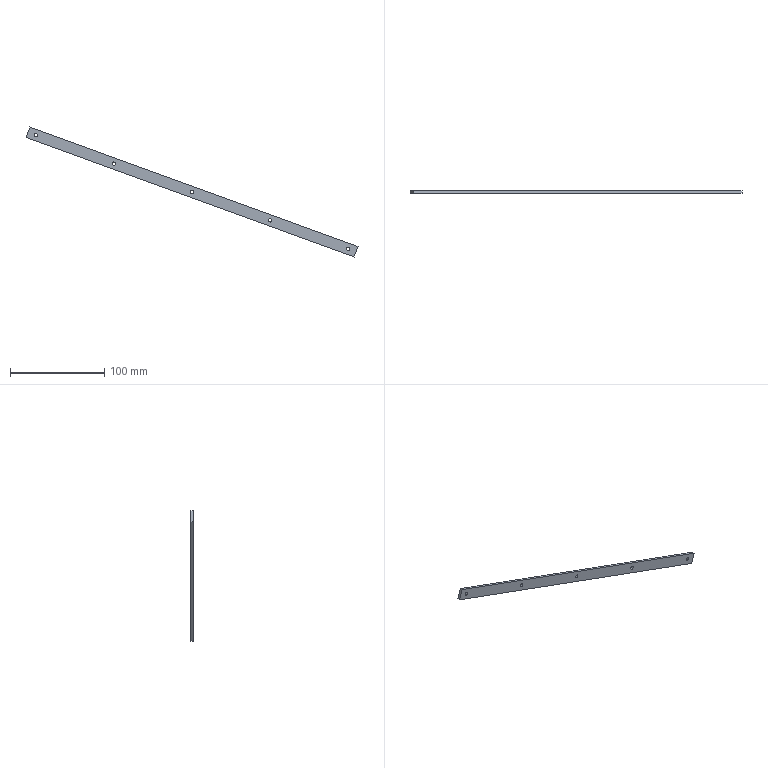Part | NX | features solid 2 | 1 solid | 16 faces | box 351.791 x 2.5 x 137.824 mm | volume 10983 mm3 | cylinder 10 | plane 6 | commonest cylinder face diameters 3.459 x10
STEP:
#1=CARTESIAN_POINT('',(-5.815,-657.5,738.773));
#2=VERTEX_POINT('',#1);
#3=CARTESIAN_POINT('',(-5.815,-655.,738.773));
#4=VERTEX_POINT('',#3);
#5=CARTESIAN_POINT('',(-5.815,-1025.203,738.773));
#6=DIRECTION('',(0.,1.,0.));
#7=VECTOR('',#6,1000.);
#8=LINE('',#5,#7);
#9=EDGE_CURVE('',#2,#4,#8,.T.);
#10=ORIENTED_EDGE('',*,*,#9,.F.);
#11=CARTESIAN_POINT('',(-9.065,-657.5,739.956));
#12=VERTEX_POINT('',#11);
#13=CARTESIAN_POINT('',(-7.44,-657.5,739.364));
#14=DIRECTION('',(0.,1.,0.));
#15=DIRECTION('',(-0.9397,0.,0.342));
#16=AXIS2_PLACEMENT_3D('',#13,#14,#15);
#17=CIRCLE('',#16,1.73);
#18=EDGE_CURVE('',#12,#2,#17,.T.);
#19=ORIENTED_EDGE('',*,*,#18,.F.);
#20=CARTESIAN_POINT('',(-9.065,-655.,739.956));
#21=VERTEX_POINT('',#20);
#22=CARTESIAN_POINT('',(-9.065,-1025.203,739.956));
#23=DIRECTION('',(0.,1.,0.));
#24=VECTOR('',#23,1000.);
#25=LINE('',#22,#24);
#26=EDGE_CURVE('',#21,#12,#25,.F.);
#27=ORIENTED_EDGE('',*,*,#26,.F.);
#28=CARTESIAN_POINT('',(-7.44,-655.,739.364));
#29=DIRECTION('',(0.,1.,0.));
#30=DIRECTION('',(-0.9397,0.,0.342));
#31=AXIS2_PLACEMENT_3D('',#28,#29,#30);
#32=CIRCLE('',#31,1.73);
#33=EDGE_CURVE('',#21,#4,#32,.T.);
#34=ORIENTED_EDGE('',*,*,#33,.T.);
#35=EDGE_LOOP('',(#10,#19,#27,#34));
#36=FACE_BOUND('',#35,.T.);
#37=CARTESIAN_POINT('',(-7.44,-1025.203,739.364));
#38=DIRECTION('',(0.,1.,0.));
#39=DIRECTION('',(-0.9397,0.,0.342));
#40=AXIS2_PLACEMENT_3D('',#37,#38,#39);
#41=CYLINDRICAL_SURFACE('',#40,1.73);
#42=ADVANCED_FACE('',(#36),#41,.F.);
#43=CARTESIAN_POINT('',(324.957,-655.,618.382));
#44=VERTEX_POINT('',#43);
#45=CARTESIAN_POINT('',(324.957,-657.5,618.382));
#46=VERTEX_POINT('',#45);
#47=CARTESIAN_POINT('',(324.957,-1025.203,618.382));
#48=DIRECTION('',(0.,1.,0.));
#49=VECTOR('',#48,1000.);
#50=LINE('',#47,#49);
#51=EDGE_CURVE('',#44,#46,#50,.F.);
#52=ORIENTED_EDGE('',*,*,#51,.T.);
#53=CARTESIAN_POINT('',(321.706,-657.5,619.565));
#54=VERTEX_POINT('',#53);
#55=CARTESIAN_POINT('',(323.332,-657.5,618.973));
#56=DIRECTION('',(0.,1.,0.));
#57=DIRECTION('',(-0.9397,0.,0.342));
#58=AXIS2_PLACEMENT_3D('',#55,#56,#57);
#59=CIRCLE('',#58,1.73);
#60=EDGE_CURVE('',#54,#46,#59,.T.);
#61=ORIENTED_EDGE('',*,*,#60,.F.);
#62=CARTESIAN_POINT('',(321.706,-655.,619.565));
#63=VERTEX_POINT('',#62);
#64=CARTESIAN_POINT('',(321.706,-1025.203,619.565));
#65=DIRECTION('',(0.,1.,0.));
#66=VECTOR('',#65,1000.);
#67=LINE('',#64,#66);
#68=EDGE_CURVE('',#54,#63,#67,.T.);
#69=ORIENTED_EDGE('',*,*,#68,.T.);
#70=CARTESIAN_POINT('',(323.332,-655.,618.973));
#71=DIRECTION('',(0.,1.,0.));
#72=DIRECTION('',(-0.9397,0.,0.342));
#73=AXIS2_PLACEMENT_3D('',#70,#71,#72);
#74=CIRCLE('',#73,1.73);
#75=EDGE_CURVE('',#63,#44,#74,.T.);
#76=ORIENTED_EDGE('',*,*,#75,.T.);
#77=EDGE_LOOP('',(#52,#61,#69,#76));
#78=FACE_BOUND('',#77,.T.);
#79=CARTESIAN_POINT('',(323.332,-1025.203,618.973));
#80=DIRECTION('',(0.,1.,0.));
#81=DIRECTION('',(-0.9397,0.,0.342));
#82=AXIS2_PLACEMENT_3D('',#79,#80,#81);
#83=CYLINDRICAL_SURFACE('',#82,1.73);
#84=ADVANCED_FACE('',(#78),#83,.F.);
#85=CARTESIAN_POINT('',(159.571,-655.,678.577));
#86=VERTEX_POINT('',#85);
#87=CARTESIAN_POINT('',(159.571,-657.5,678.577));
#88=VERTEX_POINT('',#87);
#89=CARTESIAN_POINT('',(159.571,-1025.203,678.577));
#90=DIRECTION('',(0.,1.,0.));
#91=VECTOR('',#90,1000.);
#92=LINE('',#89,#91);
#93=EDGE_CURVE('',#86,#88,#92,.F.);
#94=ORIENTED_EDGE('',*,*,#93,.T.);
#95=CARTESIAN_POINT('',(156.32,-657.5,679.76));
#96=VERTEX_POINT('',#95);
#97=CARTESIAN_POINT('',(157.946,-657.5,679.169));
#98=DIRECTION('',(0.,1.,0.));
#99=DIRECTION('',(-0.9397,0.,0.342));
#100=AXIS2_PLACEMENT_3D('',#97,#98,#99);
#101=CIRCLE('',#100,1.73);
#102=EDGE_CURVE('',#96,#88,#101,.T.);
#103=ORIENTED_EDGE('',*,*,#102,.F.);
#104=CARTESIAN_POINT('',(156.32,-655.,679.76));
#105=VERTEX_POINT('',#104);
#106=CARTESIAN_POINT('',(156.32,-1025.203,679.76));
#107=DIRECTION('',(0.,1.,0.));
#108=VECTOR('',#107,1000.);
#109=LINE('',#106,#108);
#110=EDGE_CURVE('',#96,#105,#109,.T.);
#111=ORIENTED_EDGE('',*,*,#110,.T.);
#112=CARTESIAN_POINT('',(157.946,-655.,679.169));
#113=DIRECTION('',(0.,1.,0.));
#114=DIRECTION('',(-0.9397,0.,0.342));
#115=AXIS2_PLACEMENT_3D('',#112,#113,#114);
#116=CIRCLE('',#115,1.73);
#117=EDGE_CURVE('',#105,#86,#116,.T.);
#118=ORIENTED_EDGE('',*,*,#117,.T.);
#119=EDGE_LOOP('',(#94,#103,#111,#118));
#120=FACE_BOUND('',#119,.T.);
#121=CARTESIAN_POINT('',(157.946,-1025.203,679.169));
#122=DIRECTION('',(0.,1.,0.));
#123=DIRECTION('',(-0.9397,0.,0.342));
#124=AXIS2_PLACEMENT_3D('',#121,#122,#123);
#125=CYLINDRICAL_SURFACE('',#124,1.73);
#126=ADVANCED_FACE('',(#120),#125,.F.);
#127=CARTESIAN_POINT('',(76.878,-657.5,708.675));
#128=VERTEX_POINT('',#127);
#129=CARTESIAN_POINT('',(76.878,-655.,708.675));
#130=VERTEX_POINT('',#129);
#131=CARTESIAN_POINT('',(76.878,-1025.203,708.675));
#132=DIRECTION('',(0.,1.,0.));
#133=VECTOR('',#132,1000.);
#134=LINE('',#131,#133);
#135=EDGE_CURVE('',#128,#130,#134,.T.);
#136=ORIENTED_EDGE('',*,*,#135,.F.);
#137=CARTESIAN_POINT('',(73.628,-657.5,709.858));
#138=VERTEX_POINT('',#137);
#139=CARTESIAN_POINT('',(75.253,-657.5,709.267));
#140=DIRECTION('',(0.,1.,0.));
#141=DIRECTION('',(-0.9397,0.,0.342));
#142=AXIS2_PLACEMENT_3D('',#139,#140,#141);
#143=CIRCLE('',#142,1.73);
#144=EDGE_CURVE('',#138,#128,#143,.T.);
#145=ORIENTED_EDGE('',*,*,#144,.F.);
#146=CARTESIAN_POINT('',(73.628,-655.,709.858));
#147=VERTEX_POINT('',#146);
#148=CARTESIAN_POINT('',(73.628,-1025.203,709.858));
#149=DIRECTION('',(0.,1.,0.));
#150=VECTOR('',#149,1000.);
#151=LINE('',#148,#150);
#152=EDGE_CURVE('',#147,#138,#151,.F.);
#153=ORIENTED_EDGE('',*,*,#152,.F.);
#154=CARTESIAN_POINT('',(75.253,-655.,709.267));
#155=DIRECTION('',(0.,1.,0.));
#156=DIRECTION('',(-0.9397,0.,0.342));
#157=AXIS2_PLACEMENT_3D('',#154,#155,#156);
#158=CIRCLE('',#157,1.73);
#159=EDGE_CURVE('',#147,#130,#158,.T.);
#160=ORIENTED_EDGE('',*,*,#159,.T.);
#161=EDGE_LOOP('',(#136,#145,#153,#160));
#162=FACE_BOUND('',#161,.T.);
#163=CARTESIAN_POINT('',(75.253,-1025.203,709.267));
#164=DIRECTION('',(0.,1.,0.));
#165=DIRECTION('',(-0.9397,0.,0.342));
#166=AXIS2_PLACEMENT_3D('',#163,#164,#165);
#167=CYLINDRICAL_SURFACE('',#166,1.73);
#168=ADVANCED_FACE('',(#162),#167,.F.);
#169=CARTESIAN_POINT('',(242.264,-657.5,648.48));
#170=VERTEX_POINT('',#169);
#171=CARTESIAN_POINT('',(242.264,-655.,648.48));
#172=VERTEX_POINT('',#171);
#173=CARTESIAN_POINT('',(242.264,-1025.203,648.48));
#174=DIRECTION('',(0.,1.,0.));
#175=VECTOR('',#174,1000.);
#176=LINE('',#173,#175);
#177=EDGE_CURVE('',#170,#172,#176,.T.);
#178=ORIENTED_EDGE('',*,*,#177,.F.);
#179=CARTESIAN_POINT('',(239.013,-657.5,649.663));
#180=VERTEX_POINT('',#179);
#181=CARTESIAN_POINT('',(240.639,-657.5,649.071));
#182=DIRECTION('',(0.,1.,0.));
#183=DIRECTION('',(-0.9397,0.,0.342));
#184=AXIS2_PLACEMENT_3D('',#181,#182,#183);
#185=CIRCLE('',#184,1.73);
#186=EDGE_CURVE('',#180,#170,#185,.T.);
#187=ORIENTED_EDGE('',*,*,#186,.F.);
#188=CARTESIAN_POINT('',(239.013,-655.,649.663));
#189=VERTEX_POINT('',#188);
#190=CARTESIAN_POINT('',(239.013,-1025.203,649.663));
#191=DIRECTION('',(0.,1.,0.));
#192=VECTOR('',#191,1000.);
#193=LINE('',#190,#192);
#194=EDGE_CURVE('',#189,#180,#193,.F.);
#195=ORIENTED_EDGE('',*,*,#194,.F.);
#196=CARTESIAN_POINT('',(240.639,-655.,649.071));
#197=DIRECTION('',(0.,1.,0.));
#198=DIRECTION('',(-0.9397,0.,0.342));
#199=AXIS2_PLACEMENT_3D('',#196,#197,#198);
#200=CIRCLE('',#199,1.73);
#201=EDGE_CURVE('',#189,#172,#200,.T.);
#202=ORIENTED_EDGE('',*,*,#201,.T.);
#203=EDGE_LOOP('',(#178,#187,#195,#202));
#204=FACE_BOUND('',#203,.T.);
#205=CARTESIAN_POINT('',(240.639,-1025.203,649.071));
#206=DIRECTION('',(0.,1.,0.));
#207=DIRECTION('',(-0.9397,0.,0.342));
#208=AXIS2_PLACEMENT_3D('',#205,#206,#207);
#209=CYLINDRICAL_SURFACE('',#208,1.73);
#210=ADVANCED_FACE('',(#204),#209,.F.);
#211=ORIENTED_EDGE('',*,*,#201,.F.);
#212=CARTESIAN_POINT('',(240.639,-655.,649.071));
#213=DIRECTION('',(0.,1.,0.));
#214=DIRECTION('',(-0.9397,0.,0.342));
#215=AXIS2_PLACEMENT_3D('',#212,#213,#214);
#216=CIRCLE('',#215,1.73);
#217=EDGE_CURVE('',#172,#189,#216,.T.);
#218=ORIENTED_EDGE('',*,*,#217,.F.);
#219=EDGE_LOOP('',(#211,#218));
#220=FACE_BOUND('',#219,.T.);
#221=ORIENTED_EDGE('',*,*,#159,.F.);
#222=CARTESIAN_POINT('',(75.253,-655.,709.267));
#223=DIRECTION('',(0.,1.,0.));
#224=DIRECTION('',(-0.9397,0.,0.342));
#225=AXIS2_PLACEMENT_3D('',#222,#223,#224);
#226=CIRCLE('',#225,1.73);
#227=EDGE_CURVE('',#130,#147,#226,.T.);
#228=ORIENTED_EDGE('',*,*,#227,.F.);
#229=EDGE_LOOP('',(#221,#228));
#230=FACE_BOUND('',#229,.T.);
#231=ORIENTED_EDGE('',*,*,#117,.F.);
#232=CARTESIAN_POINT('',(157.946,-655.,679.169));
#233=DIRECTION('',(0.,1.,0.));
#234=DIRECTION('',(-0.9397,0.,0.342));
#235=AXIS2_PLACEMENT_3D('',#232,#233,#234);
#236=CIRCLE('',#235,1.73);
#237=EDGE_CURVE('',#86,#105,#236,.T.);
#238=ORIENTED_EDGE('',*,*,#237,.F.);
#239=EDGE_LOOP('',(#231,#238));
#240=FACE_BOUND('',#239,.T.);
#241=ORIENTED_EDGE('',*,*,#75,.F.);
#242=CARTESIAN_POINT('',(323.332,-655.,618.973));
#243=DIRECTION('',(0.,1.,0.));
#244=DIRECTION('',(-0.9397,0.,0.342));
#245=AXIS2_PLACEMENT_3D('',#242,#243,#244);
#246=CIRCLE('',#245,1.73);
#247=EDGE_CURVE('',#44,#63,#246,.T.);
#248=ORIENTED_EDGE('',*,*,#247,.F.);
#249=EDGE_LOOP('',(#241,#248));
#250=FACE_BOUND('',#249,.T.);
#251=ORIENTED_EDGE('',*,*,#33,.F.);
#252=CARTESIAN_POINT('',(-7.44,-655.,739.364));
#253=DIRECTION('',(0.,1.,0.));
#254=DIRECTION('',(-0.9397,0.,0.342));
#255=AXIS2_PLACEMENT_3D('',#252,#253,#254);
#256=CIRCLE('',#255,1.73);
#257=EDGE_CURVE('',#4,#21,#256,.T.);
#258=ORIENTED_EDGE('',*,*,#257,.F.);
#259=EDGE_LOOP('',(#251,#258));
#260=FACE_BOUND('',#259,.T.);
#261=CARTESIAN_POINT('',(-17.95,-655.,736.804));
#262=VERTEX_POINT('',#261);
#263=CARTESIAN_POINT('',(-13.845,-655.,748.081));
#264=VERTEX_POINT('',#263);
#265=CARTESIAN_POINT('',(-17.95,-655.,736.804));
#266=DIRECTION('',(0.342,0.,0.9397));
#267=VECTOR('',#266,1000.);
#268=LINE('',#265,#267);
#269=EDGE_CURVE('',#262,#264,#268,.T.);
#270=ORIENTED_EDGE('',*,*,#269,.T.);
#271=CARTESIAN_POINT('',(333.841,-655.,621.533));
#272=VERTEX_POINT('',#271);
#273=CARTESIAN_POINT('',(-13.845,-655.,748.081));
#274=DIRECTION('',(0.9397,0.,-0.342));
#275=VECTOR('',#274,1000.);
#276=LINE('',#273,#275);
#277=EDGE_CURVE('',#264,#272,#276,.T.);
#278=ORIENTED_EDGE('',*,*,#277,.T.);
#279=CARTESIAN_POINT('',(329.737,-655.,610.257));
#280=VERTEX_POINT('',#279);
#281=CARTESIAN_POINT('',(329.737,-655.,610.257));
#282=DIRECTION('',(-0.342,0.,-0.9397));
#283=VECTOR('',#282,1000.);
#284=LINE('',#281,#283);
#285=EDGE_CURVE('',#272,#280,#284,.T.);
#286=ORIENTED_EDGE('',*,*,#285,.T.);
#287=CARTESIAN_POINT('',(-17.95,-655.,736.804));
#288=DIRECTION('',(-0.9397,0.,0.342));
#289=VECTOR('',#288,1000.);
#290=LINE('',#287,#289);
#291=EDGE_CURVE('',#280,#262,#290,.T.);
#292=ORIENTED_EDGE('',*,*,#291,.T.);
#293=EDGE_LOOP('',(#270,#278,#286,#292));
#294=FACE_BOUND('',#293,.T.);
#295=CARTESIAN_POINT('',(157.946,-655.,679.169));
#296=DIRECTION('',(0.,1.,0.));
#297=DIRECTION('',(0.,0.,-1.));
#298=AXIS2_PLACEMENT_3D('',#295,#296,#297);
#299=PLANE('',#298);
#300=ADVANCED_FACE('',(#220,#230,#240,#250,#260,#294),#299,.T.);
#301=ORIENTED_EDGE('',*,*,#186,.T.);
#302=CARTESIAN_POINT('',(240.639,-657.5,649.071));
#303=DIRECTION('',(0.,1.,0.));
#304=DIRECTION('',(-0.9397,0.,0.342));
#305=AXIS2_PLACEMENT_3D('',#302,#303,#304);
#306=CIRCLE('',#305,1.73);
#307=EDGE_CURVE('',#170,#180,#306,.T.);
#308=ORIENTED_EDGE('',*,*,#307,.T.);
#309=EDGE_LOOP('',(#301,#308));
#310=FACE_BOUND('',#309,.T.);
#311=ORIENTED_EDGE('',*,*,#144,.T.);
#312=CARTESIAN_POINT('',(75.253,-657.5,709.267));
#313=DIRECTION('',(0.,1.,0.));
#314=DIRECTION('',(-0.9397,0.,0.342));
#315=AXIS2_PLACEMENT_3D('',#312,#313,#314);
#316=CIRCLE('',#315,1.73);
#317=EDGE_CURVE('',#128,#138,#316,.T.);
#318=ORIENTED_EDGE('',*,*,#317,.T.);
#319=EDGE_LOOP('',(#311,#318));
#320=FACE_BOUND('',#319,.T.);
#321=ORIENTED_EDGE('',*,*,#102,.T.);
#322=CARTESIAN_POINT('',(157.946,-657.5,679.169));
#323=DIRECTION('',(0.,1.,0.));
#324=DIRECTION('',(-0.9397,0.,0.342));
#325=AXIS2_PLACEMENT_3D('',#322,#323,#324);
#326=CIRCLE('',#325,1.73);
#327=EDGE_CURVE('',#88,#96,#326,.T.);
#328=ORIENTED_EDGE('',*,*,#327,.T.);
#329=EDGE_LOOP('',(#321,#328));
#330=FACE_BOUND('',#329,.T.);
#331=ORIENTED_EDGE('',*,*,#60,.T.);
#332=CARTESIAN_POINT('',(323.332,-657.5,618.973));
#333=DIRECTION('',(0.,1.,0.));
#334=DIRECTION('',(-0.9397,0.,0.342));
#335=AXIS2_PLACEMENT_3D('',#332,#333,#334);
#336=CIRCLE('',#335,1.73);
#337=EDGE_CURVE('',#46,#54,#336,.T.);
#338=ORIENTED_EDGE('',*,*,#337,.T.);
#339=EDGE_LOOP('',(#331,#338));
#340=FACE_BOUND('',#339,.T.);
#341=ORIENTED_EDGE('',*,*,#18,.T.);
#342=CARTESIAN_POINT('',(-7.44,-657.5,739.364));
#343=DIRECTION('',(0.,1.,0.));
#344=DIRECTION('',(-0.9397,0.,0.342));
#345=AXIS2_PLACEMENT_3D('',#342,#343,#344);
#346=CIRCLE('',#345,1.73);
#347=EDGE_CURVE('',#2,#12,#346,.T.);
#348=ORIENTED_EDGE('',*,*,#347,.T.);
#349=EDGE_LOOP('',(#341,#348));
#350=FACE_BOUND('',#349,.T.);
#351=CARTESIAN_POINT('',(-17.95,-657.5,736.804));
#352=VERTEX_POINT('',#351);
#353=CARTESIAN_POINT('',(-13.845,-657.5,748.081));
#354=VERTEX_POINT('',#353);
#355=CARTESIAN_POINT('',(-17.95,-657.5,736.804));
#356=DIRECTION('',(0.342,0.,0.9397));
#357=VECTOR('',#356,1000.);
#358=LINE('',#355,#357);
#359=EDGE_CURVE('',#352,#354,#358,.T.);
#360=ORIENTED_EDGE('',*,*,#359,.F.);
#361=CARTESIAN_POINT('',(329.737,-657.5,610.257));
#362=VERTEX_POINT('',#361);
#363=CARTESIAN_POINT('',(-17.95,-657.5,736.804));
#364=DIRECTION('',(-0.9397,0.,0.342));
#365=VECTOR('',#364,1000.);
#366=LINE('',#363,#365);
#367=EDGE_CURVE('',#362,#352,#366,.T.);
#368=ORIENTED_EDGE('',*,*,#367,.F.);
#369=CARTESIAN_POINT('',(333.841,-657.5,621.533));
#370=VERTEX_POINT('',#369);
#371=CARTESIAN_POINT('',(329.737,-657.5,610.257));
#372=DIRECTION('',(-0.342,0.,-0.9397));
#373=VECTOR('',#372,1000.);
#374=LINE('',#371,#373);
#375=EDGE_CURVE('',#370,#362,#374,.T.);
#376=ORIENTED_EDGE('',*,*,#375,.F.);
#377=CARTESIAN_POINT('',(-13.845,-657.5,748.081));
#378=DIRECTION('',(0.9397,0.,-0.342));
#379=VECTOR('',#378,1000.);
#380=LINE('',#377,#379);
#381=EDGE_CURVE('',#354,#370,#380,.T.);
#382=ORIENTED_EDGE('',*,*,#381,.F.);
#383=EDGE_LOOP('',(#360,#368,#376,#382));
#384=FACE_BOUND('',#383,.T.);
#385=CARTESIAN_POINT('',(157.946,-657.5,679.169));
#386=DIRECTION('',(0.,1.,0.));
#387=DIRECTION('',(0.,0.,-1.));
#388=AXIS2_PLACEMENT_3D('',#385,#386,#387);
#389=PLANE('',#388);
#390=ADVANCED_FACE('',(#310,#320,#330,#340,#350,#384),#389,.F.);
#391=ORIENTED_EDGE('',*,*,#291,.F.);
#392=CARTESIAN_POINT('',(329.737,-657.5,610.257));
#393=DIRECTION('',(0.,1.,0.));
#394=VECTOR('',#393,1000.);
#395=LINE('',#392,#394);
#396=EDGE_CURVE('',#362,#280,#395,.T.);
#397=ORIENTED_EDGE('',*,*,#396,.F.);
#398=ORIENTED_EDGE('',*,*,#367,.T.);
#399=CARTESIAN_POINT('',(-17.95,-657.5,736.804));
#400=DIRECTION('',(0.,1.,0.));
#401=VECTOR('',#400,1000.);
#402=LINE('',#399,#401);
#403=EDGE_CURVE('',#352,#262,#402,.T.);
#404=ORIENTED_EDGE('',*,*,#403,.T.);
#405=EDGE_LOOP('',(#391,#397,#398,#404));
#406=FACE_BOUND('',#405,.T.);
#407=CARTESIAN_POINT('',(-17.95,-657.5,736.804));
#408=DIRECTION('',(-0.342,0.,-0.9397));
#409=DIRECTION('',(-0.9397,0.,0.342));
#410=AXIS2_PLACEMENT_3D('',#407,#408,#409);
#411=PLANE('',#410);
#412=ADVANCED_FACE('',(#406),#411,.T.);
#413=ORIENTED_EDGE('',*,*,#285,.F.);
#414=CARTESIAN_POINT('',(333.841,-657.5,621.533));
#415=DIRECTION('',(0.,1.,0.));
#416=VECTOR('',#415,1000.);
#417=LINE('',#414,#416);
#418=EDGE_CURVE('',#370,#272,#417,.T.);
#419=ORIENTED_EDGE('',*,*,#418,.F.);
#420=ORIENTED_EDGE('',*,*,#375,.T.);
#421=ORIENTED_EDGE('',*,*,#396,.T.);
#422=EDGE_LOOP('',(#413,#419,#420,#421));
#423=FACE_BOUND('',#422,.T.);
#424=CARTESIAN_POINT('',(329.737,-657.5,610.257));
#425=DIRECTION('',(0.9397,0.,-0.342));
#426=DIRECTION('',(0.,-1.,0.));
#427=AXIS2_PLACEMENT_3D('',#424,#425,#426);
#428=PLANE('',#427);
#429=ADVANCED_FACE('',(#423),#428,.T.);
#430=ORIENTED_EDGE('',*,*,#277,.F.);
#431=CARTESIAN_POINT('',(-13.845,-657.5,748.081));
#432=DIRECTION('',(0.,1.,0.));
#433=VECTOR('',#432,1000.);
#434=LINE('',#431,#433);
#435=EDGE_CURVE('',#354,#264,#434,.T.);
#436=ORIENTED_EDGE('',*,*,#435,.F.);
#437=ORIENTED_EDGE('',*,*,#381,.T.);
#438=ORIENTED_EDGE('',*,*,#418,.T.);
#439=EDGE_LOOP('',(#430,#436,#437,#438));
#440=FACE_BOUND('',#439,.T.);
#441=CARTESIAN_POINT('',(-13.845,-657.5,748.081));
#442=DIRECTION('',(0.342,0.,0.9397));
#443=DIRECTION('',(0.,-1.,0.));
#444=AXIS2_PLACEMENT_3D('',#441,#442,#443);
#445=PLANE('',#444);
#446=ADVANCED_FACE('',(#440),#445,.T.);
#447=ORIENTED_EDGE('',*,*,#269,.F.);
#448=ORIENTED_EDGE('',*,*,#403,.F.);
#449=ORIENTED_EDGE('',*,*,#359,.T.);
#450=ORIENTED_EDGE('',*,*,#435,.T.);
#451=EDGE_LOOP('',(#447,#448,#449,#450));
#452=FACE_BOUND('',#451,.T.);
#453=CARTESIAN_POINT('',(-17.95,-657.5,736.804));
#454=DIRECTION('',(-0.9397,0.,0.342));
#455=DIRECTION('',(0.,1.,0.));
#456=AXIS2_PLACEMENT_3D('',#453,#454,#455);
#457=PLANE('',#456);
#458=ADVANCED_FACE('',(#452),#457,.T.);
#459=ORIENTED_EDGE('',*,*,#307,.F.);
#460=ORIENTED_EDGE('',*,*,#177,.T.);
#461=ORIENTED_EDGE('',*,*,#217,.T.);
#462=ORIENTED_EDGE('',*,*,#194,.T.);
#463=EDGE_LOOP('',(#459,#460,#461,#462));
#464=FACE_BOUND('',#463,.T.);
#465=CARTESIAN_POINT('',(240.639,-1025.203,649.071));
#466=DIRECTION('',(0.,1.,0.));
#467=DIRECTION('',(-0.9397,0.,0.342));
#468=AXIS2_PLACEMENT_3D('',#465,#466,#467);
#469=CYLINDRICAL_SURFACE('',#468,1.73);
#470=ADVANCED_FACE('',(#464),#469,.F.);
#471=ORIENTED_EDGE('',*,*,#317,.F.);
#472=ORIENTED_EDGE('',*,*,#135,.T.);
#473=ORIENTED_EDGE('',*,*,#227,.T.);
#474=ORIENTED_EDGE('',*,*,#152,.T.);
#475=EDGE_LOOP('',(#471,#472,#473,#474));
#476=FACE_BOUND('',#475,.T.);
#477=CARTESIAN_POINT('',(75.253,-1025.203,709.267));
#478=DIRECTION('',(0.,1.,0.));
#479=DIRECTION('',(-0.9397,0.,0.342));
#480=AXIS2_PLACEMENT_3D('',#477,#478,#479);
#481=CYLINDRICAL_SURFACE('',#480,1.73);
#482=ADVANCED_FACE('',(#476),#481,.F.);
#483=ORIENTED_EDGE('',*,*,#327,.F.);
#484=ORIENTED_EDGE('',*,*,#93,.F.);
#485=ORIENTED_EDGE('',*,*,#237,.T.);
#486=ORIENTED_EDGE('',*,*,#110,.F.);
#487=EDGE_LOOP('',(#483,#484,#485,#486));
#488=FACE_BOUND('',#487,.T.);
#489=CARTESIAN_POINT('',(157.946,-1025.203,679.169));
#490=DIRECTION('',(0.,1.,0.));
#491=DIRECTION('',(-0.9397,0.,0.342));
#492=AXIS2_PLACEMENT_3D('',#489,#490,#491);
#493=CYLINDRICAL_SURFACE('',#492,1.73);
#494=ADVANCED_FACE('',(#488),#493,.F.);
#495=ORIENTED_EDGE('',*,*,#337,.F.);
#496=ORIENTED_EDGE('',*,*,#51,.F.);
#497=ORIENTED_EDGE('',*,*,#247,.T.);
#498=ORIENTED_EDGE('',*,*,#68,.F.);
#499=EDGE_LOOP('',(#495,#496,#497,#498));
#500=FACE_BOUND('',#499,.T.);
#501=CARTESIAN_POINT('',(323.332,-1025.203,618.973));
#502=DIRECTION('',(0.,1.,0.));
#503=DIRECTION('',(-0.9397,0.,0.342));
#504=AXIS2_PLACEMENT_3D('',#501,#502,#503);
#505=CYLINDRICAL_SURFACE('',#504,1.73);
#506=ADVANCED_FACE('',(#500),#505,.F.);
#507=ORIENTED_EDGE('',*,*,#347,.F.);
#508=ORIENTED_EDGE('',*,*,#9,.T.);
#509=ORIENTED_EDGE('',*,*,#257,.T.);
#510=ORIENTED_EDGE('',*,*,#26,.T.);
#511=EDGE_LOOP('',(#507,#508,#509,#510));
#512=FACE_BOUND('',#511,.T.);
#513=CARTESIAN_POINT('',(-7.44,-1025.203,739.364));
#514=DIRECTION('',(0.,1.,0.));
#515=DIRECTION('',(-0.9397,0.,0.342));
#516=AXIS2_PLACEMENT_3D('',#513,#514,#515);
#517=CYLINDRICAL_SURFACE('',#516,1.73);
#518=ADVANCED_FACE('',(#512),#517,.F.);
#519=CLOSED_SHELL('',(#42,#84,#126,#168,#210,#300,#390,#412,#429,#446,#458,#470,#482,#494,#506,#518));
#520=MANIFOLD_SOLID_BREP('',#519);
#521=(LENGTH_UNIT()NAMED_UNIT(*)SI_UNIT(.MILLI.,.METRE.));
#522=UNCERTAINTY_MEASURE_WITH_UNIT(LENGTH_MEASURE(0.00001),#521,'','');
#523=(NAMED_UNIT(*)PLANE_ANGLE_UNIT()SI_UNIT($,.RADIAN.));
#524=(NAMED_UNIT(*)SI_UNIT($,.STERADIAN.)SOLID_ANGLE_UNIT());
#525=(GEOMETRIC_REPRESENTATION_CONTEXT(3)GLOBAL_UNCERTAINTY_ASSIGNED_CONTEXT((#522))GLOBAL_UNIT_ASSIGNED_CONTEXT((#521,#523,#524))REPRESENTATION_CONTEXT('',''));
#526=ADVANCED_BREP_SHAPE_REPRESENTATION('',(#520),#525);